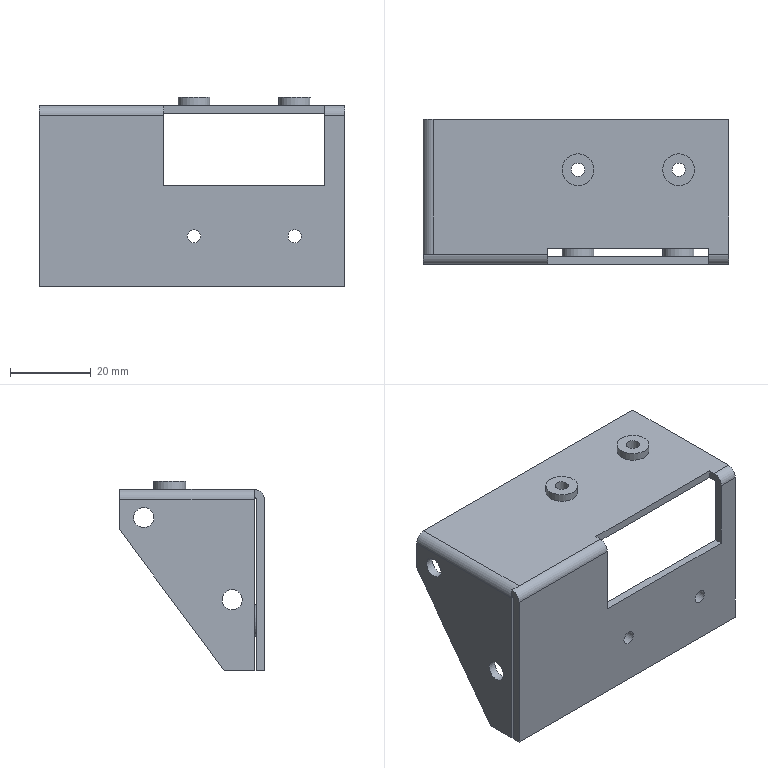Part | STEP file | 1 solid | 38 faces | box 76 x 36 x 47 mm | volume 12306 mm3 | plane 22 | cylinder 16 | commonest cylinder face diameters 5 x5 3.3 x4 7.9 x4 1 x3